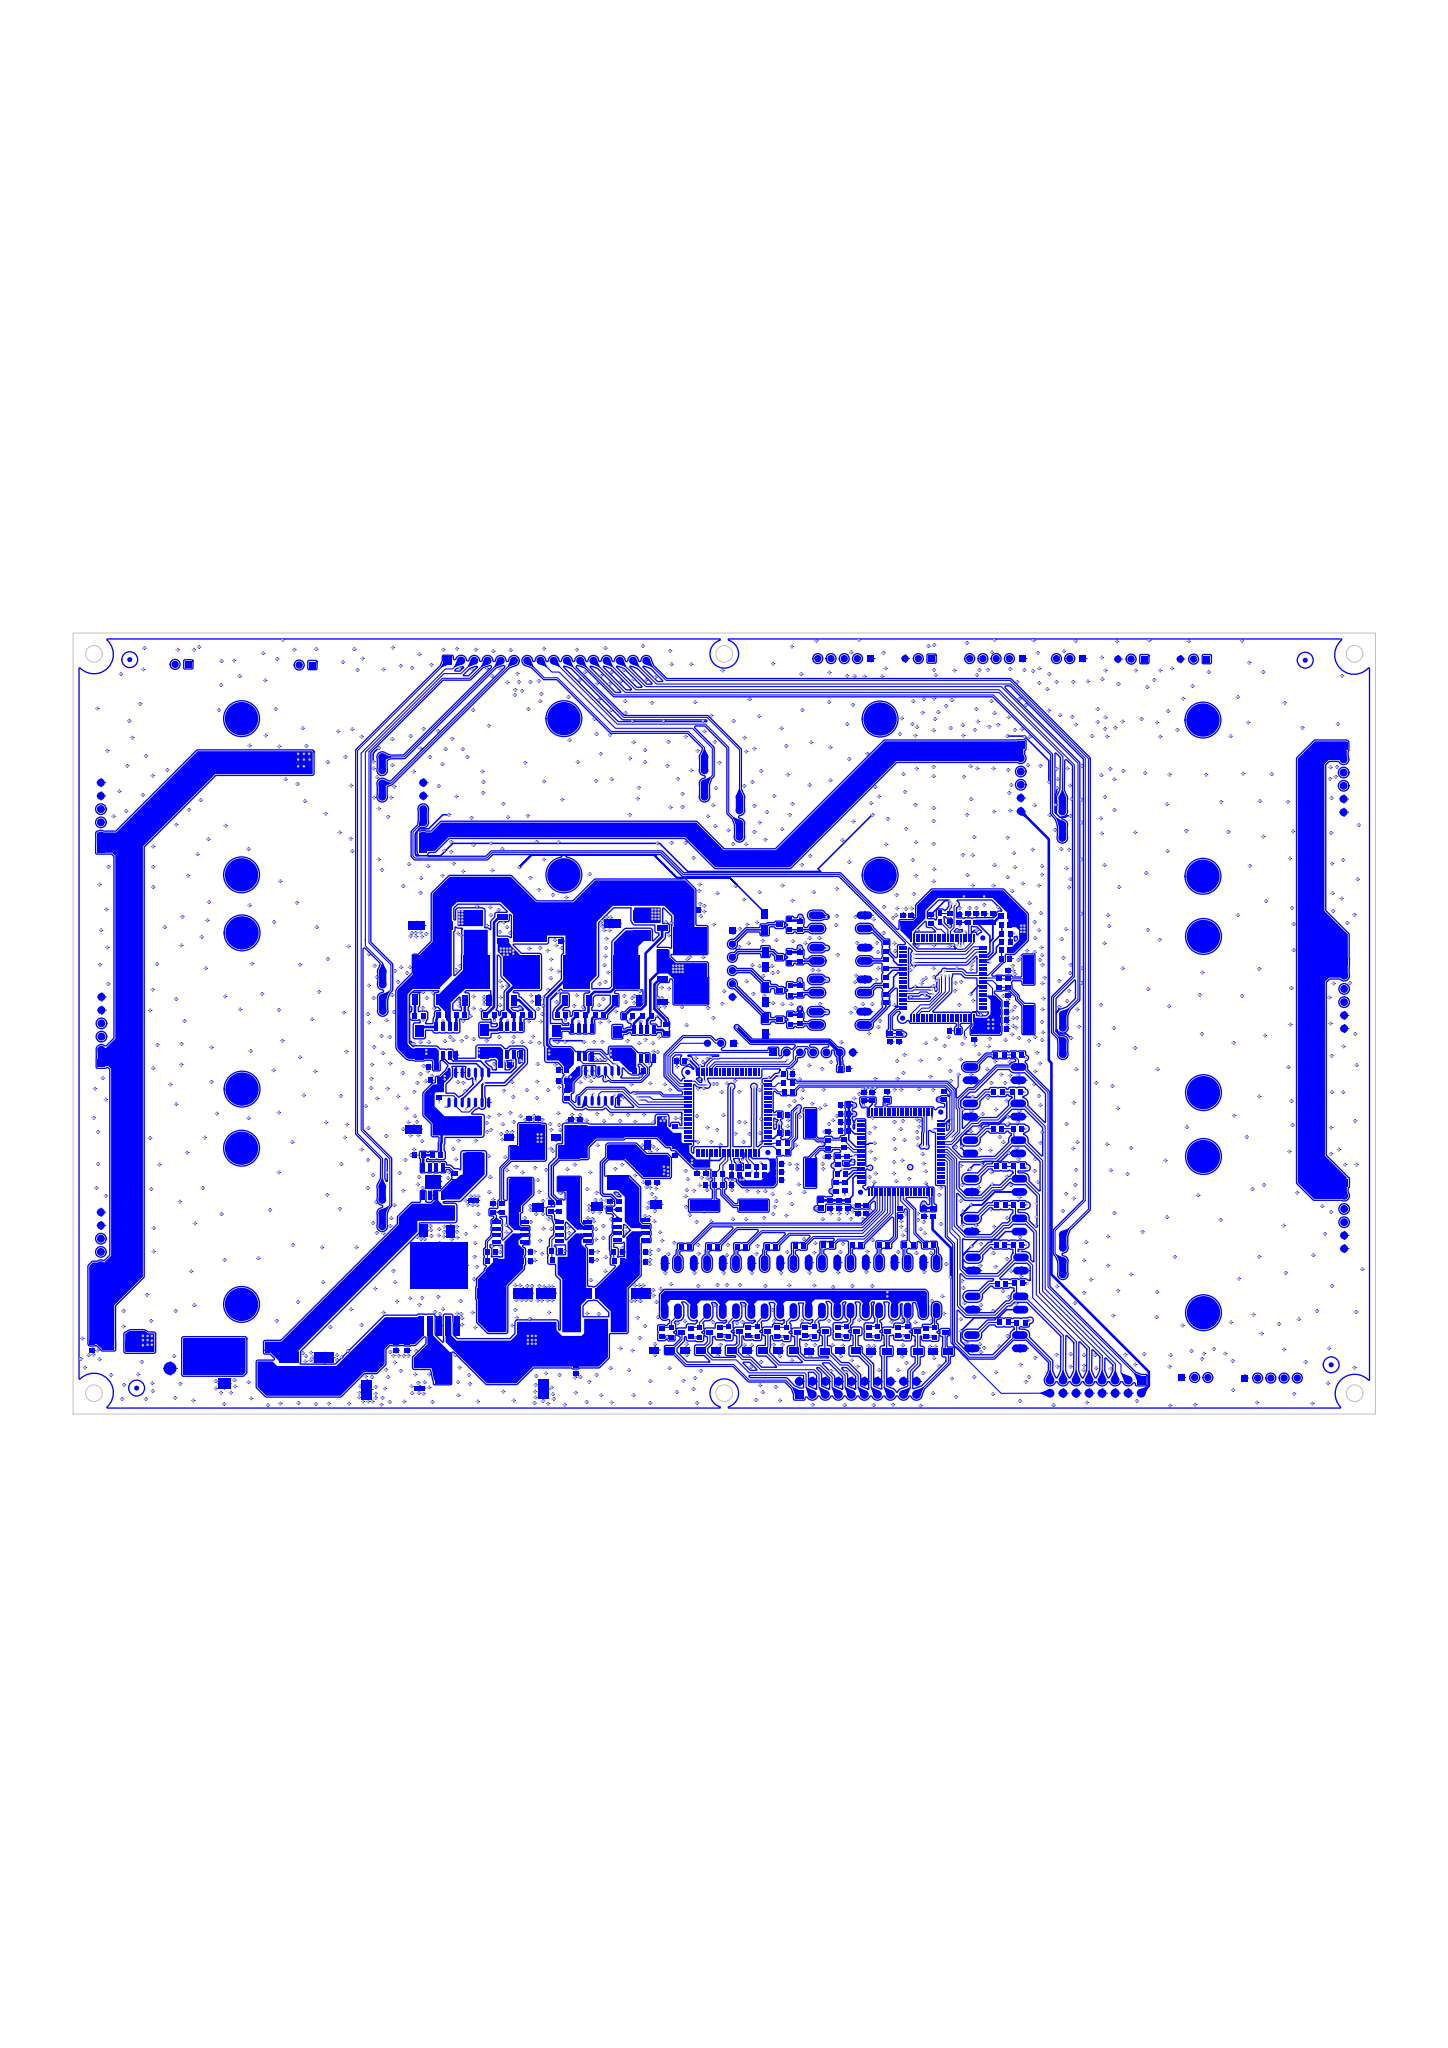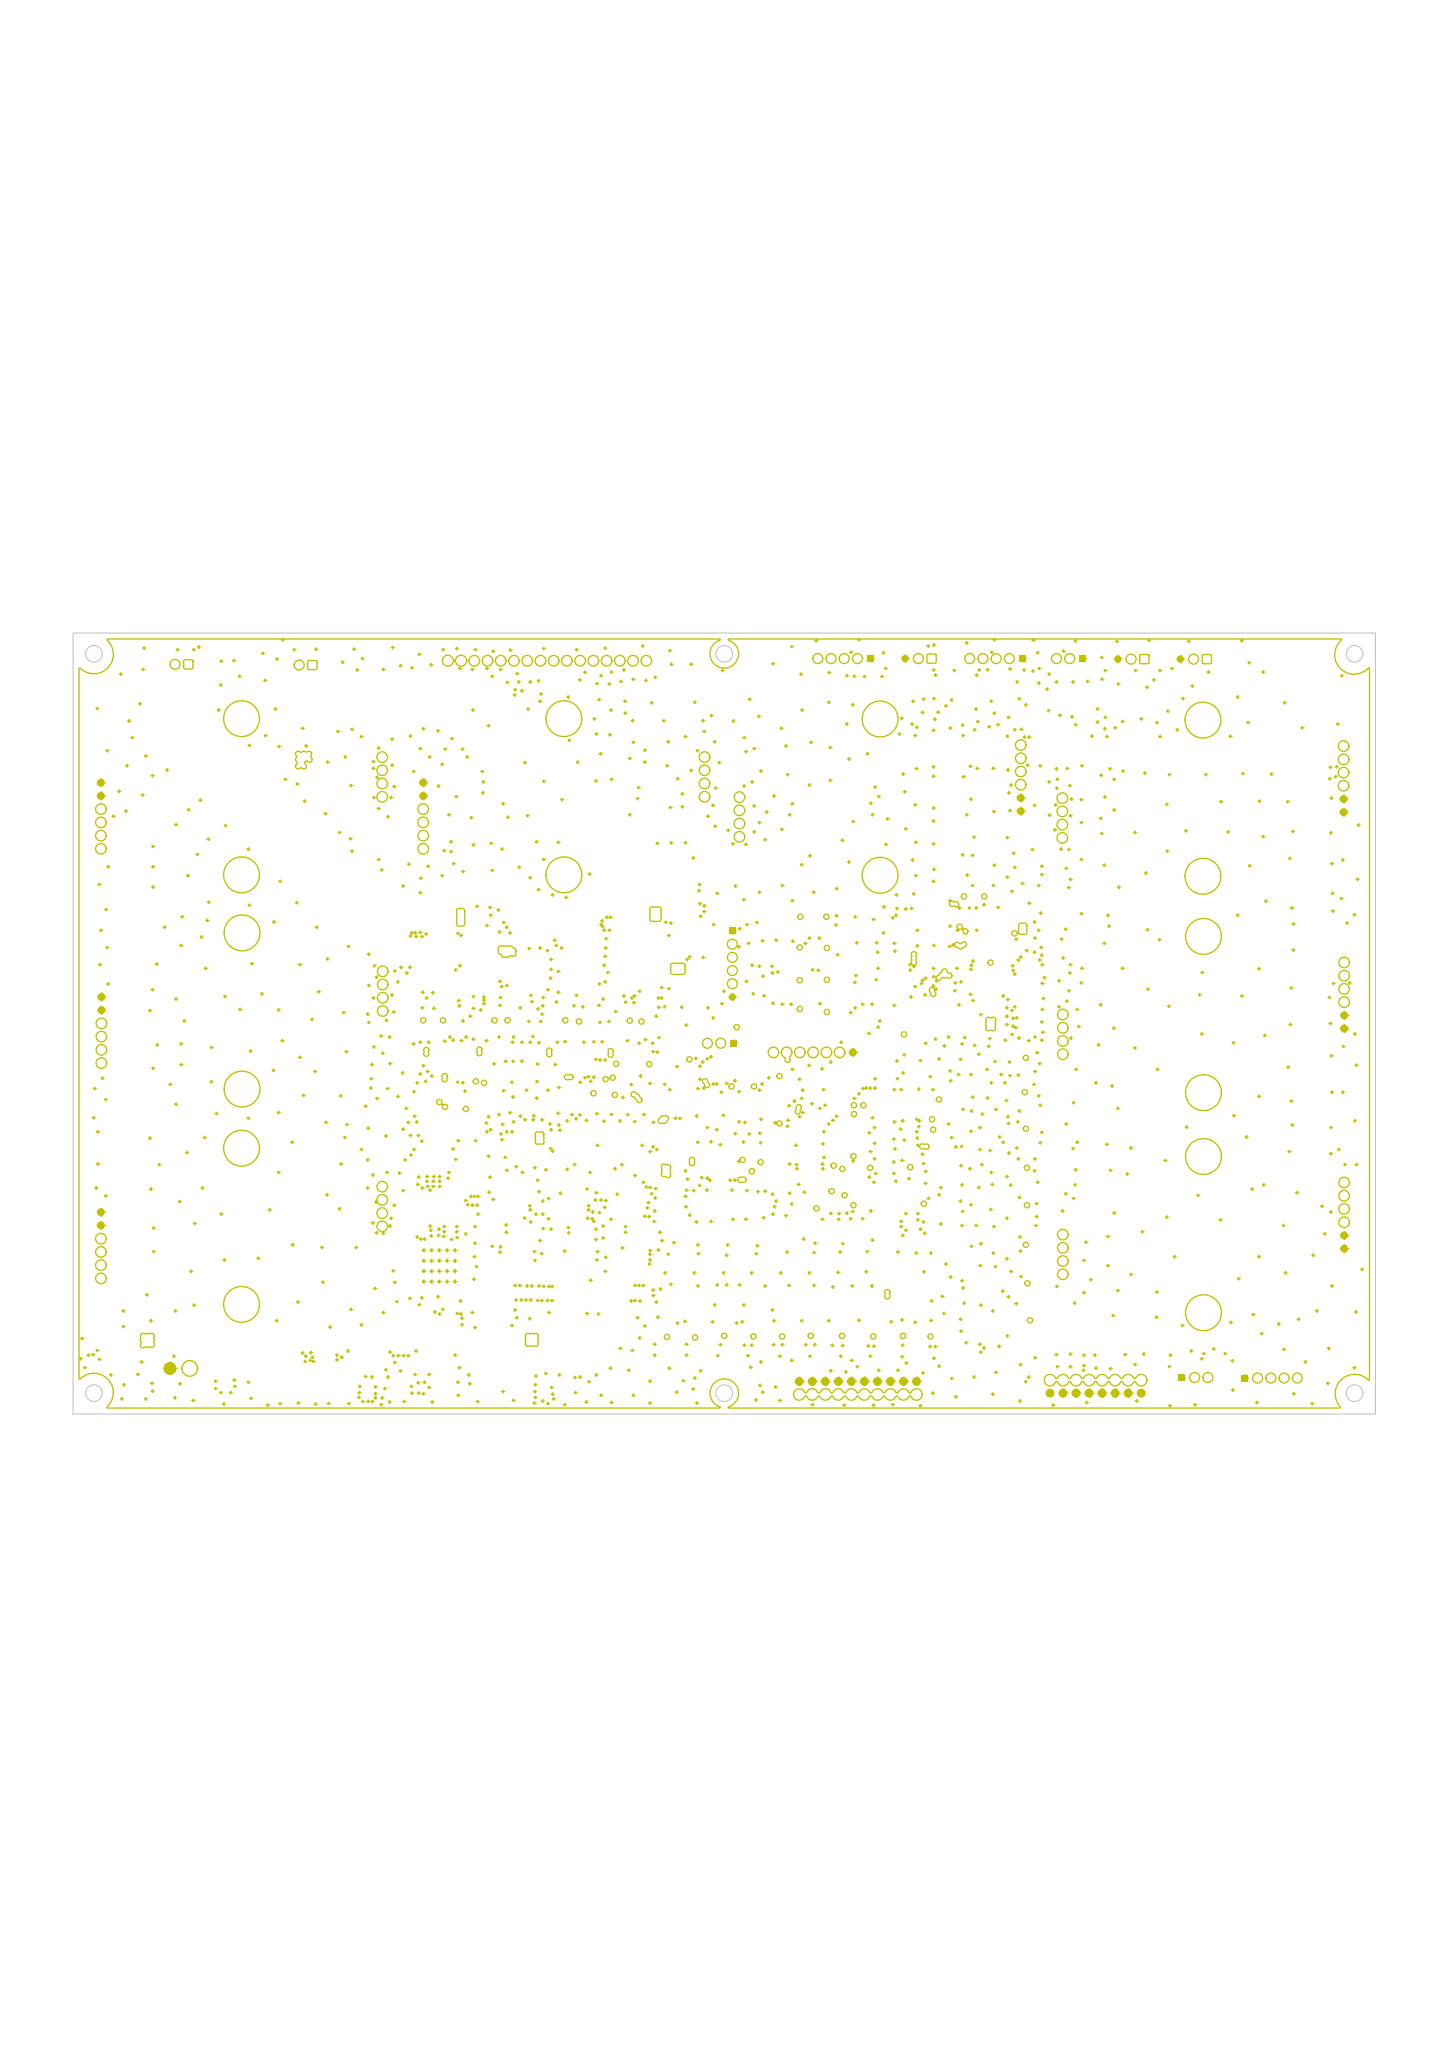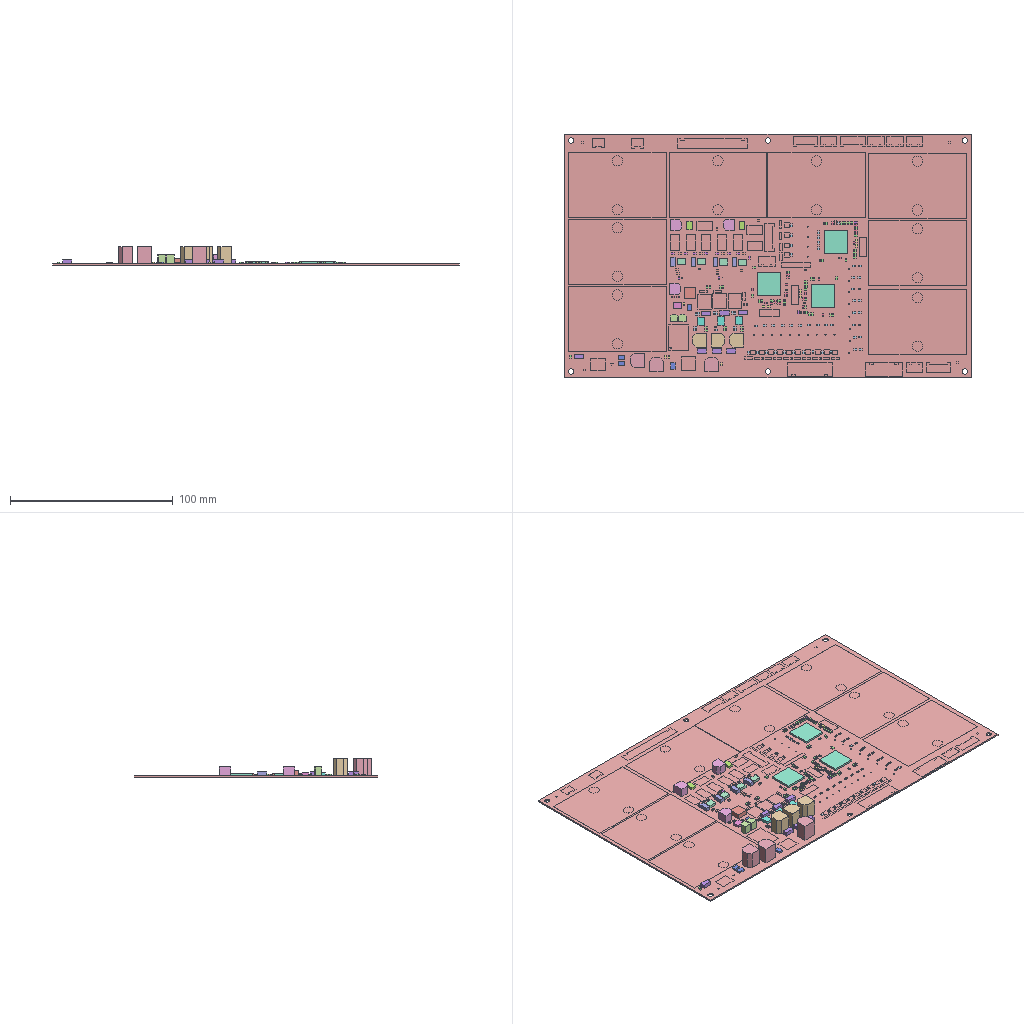Circuit board layout | Siemens PADS | box 250 x 150 x 11.4 mm
Layer stack:
layer,name,type,plane,layer_thickness_mm,copper_thickness_mm,dielectric_constant
0,,,,0,,3.3
1,Top,ROUTING,NONE,0.254,0.0343,4.3
2,Inner Layer 2,ROUTING,NONE,0.254,0.0343,4.3
3,Inner Layer 3,ROUTING,NONE,0.254,0.0343,4.3
4,Bottom,ROUTING,NONE,0,0.0343,3.3
Part placement:
Ref,PartType,Decal,X_mm,Y_mm,Rotation,Layer,Placed,Installed
C1,CAP_POL1,CAPAE830X1050N,56.395,8.15,270,Top,True,True
C2,CAP_POL1,CAPAE830X1050N,90.392,8.236,270,Top,True,True
C3,CAP_100NF_0805,C0603,110.293,45.172,90,Top,True,True
C4,CAP_100NF_0805,C0603,112.024,45.172,90,Top,True,True
C5,CAP3216,CAPAE830X1050N,82.871,23.207,0,Top,True,True
C6,CAP3216,3216,85.227,53.17,0,Top,True,True
C7,CAP_100NF_0805,C0603,89.203,55.978,270,Top,True,True
C8,CAP_100NF_0805,C0603,87.485,55.949,270,Top,True,True
C9,CAP_100NF_0805,C0603,86.921,31.17,180,Top,True,True
C10,CAP_100NF_0805,C0603,86.942,29.308,180,Top,True,True
C11,CAP3216,CAPAE830X1050N,94.232,23.207,180,Top,True,True
C12,CAP3216,3216,94.206,53.039,0,Top,True,True
C13,CAP_100NF_0805,C0603,97.278,55.851,270,Top,True,True
C14,CAP_100NF_0805,C0603,95.655,55.851,270,Top,True,True
C15,CAP_100NF_0805,C0603,98.736,31.121,180,Top,True,True
C16,CAP_100NF_0805,C0603,98.724,29.494,180,Top,True,True
C17,CAP_100NF_0805,C0603,131.981,47.469,0,Top,True,True
C18,CAP,C0603,61.963,13.017,90,Top,True,True
C19,CAP,C0603,64.165,12.988,90,Top,True,True
C20,CAP,C0603,96.464,8.581,90,Top,True,True
C21,CAP3216,CAPAE830X1050N,105.588,23.231,0,Top,True,True
C22,CAP_100NF_0805,C0603,109.049,29.24,180,Top,True,True
C23,CAP_100NF_0805,C0603,109.049,31.131,180,Top,True,True
C24,CAP3216,3216,110.244,50.174,270,Top,True,True
C25,CAP,C0603,73.389,45.447,90,Top,True,True
C26,CAP_POL1,CAPAE430X550N,72.408,36.917,270,Top,True,True
C27,CAP_POL1,CAPAE430X550N,67.231,36.99,270,Top,True,True
C28,CAP_POL1,CAPAE660X550N,68.037,54.705,180,Top,True,True
C29,CAP_100NF_0805,C0603,148.108,59.271,0,Top,True,True
C30,CAP_100NF_0805,C0603,151.754,60.975,270,Top,True,True
C31,CAP_100NF_0805,C0603,148.117,56.005,0,Top,True,True
C32,CAP_100NF_0805,C0603,164.982,38.757,90,Top,True,True
C33,CAP_100NF_0805,C0603,152.221,39.272,90,Top,True,True
C34,CAP_100NF_0805,C0603,178.382,78.817,180,Top,True,True
C35,CAP_100NF_0805,C0603,178.382,77.19,180,Top,True,True
C36,CAP_100NF_0805,C0603,170.139,95.232,270,Top,True,True
C37,CAP_100NF_0805,C0603,156.888,72.256,90,Top,True,True
C38,CAP_100NF_0805,C0603,160.932,95.012,270,Top,True,True
C39,CAP_100NF_0805,C0603,148.079,66.351,180,Top,True,True
C40,CAP_100NF_0805,C0603,115.49,50.503,90,Top,True,True
C41,CAP_100NF_0805,C0603,121.404,47.068,90,Top,True,True
C42,CAP_100NF_0805,C0603,119.71,47.068,270,Top,True,True
C43,CAP_POL1,CAPAE830X1050N,44.8,10.8,0,Top,True,True
C44,CAP_100NF_0805,C0603,3.695,12.993,90,Top,True,True
C45,CAP,C0603,122.275,43.938,180,Top,True,True
C46,CAP_POL1,CAPAE660X550N,68.679,93.81,180,Top,True,True
C47,CAPACITOR_ST,C0603,71.026,76.584,0,Top,True,True
C48,CAP,C0603,125.511,43.934,0,Top,True,True
C49,CAPACITOR_ST,C0603,83.688,76.637,180,Top,True,True
C50,CAPACITOR_ST,C0603,68.944,66.651,0,Top,True,True
C51,CAPACITOR_ST,C0603,82.895,66.941,180,Top,True,True
C52,CAP_100NF_0805,C0603,127.218,47.483,180,Top,True,True
C53,CAPACITOR_ST,C0603,93.7,91.6,270,Top,True,True
C54,CAP_100NF_0805,C0603,116.614,67.895,0,Top,True,True
C55,CAP_100NF_0805,C0603,135.183,48.075,180,Top,True,True
C56,CAP_100NF_0805,C0603,135.176,46.501,180,Top,True,True
C57,CAP_100NF_0805,C0603,135.166,44.932,180,Top,True,True
C58,CAP_100NF_0805,C0603,136.354,54.019,180,Top,True,True
C59,CAPACITOR_ST,C0603,69.486,64.112,180,Top,True,True
C60,CAP_POL1,CAPAE660X550N,100.794,94.206,0,Top,True,True
C61,CAPACITOR_ST,C0603,97.529,76.62,0,Top,True,True
C62,CAPACITOR_ST,C0603,110.153,76.424,180,Top,True,True
C63,CAPACITOR_ST,C0603,93.982,66.145,0,Top,True,True
C64,CAP_100NF_0805,C0603,137.211,65.229,180,Top,True,True
C65,CAPACITOR_ST,C0603,108.662,65.975,180,Top,True,True
C66,CAPACITOR_ST,C0603,119.2,96.8,0,Top,True,True
C67,CAPACITOR_ST,C0603,93.903,63.946,180,Top,True,True
C68,CAP3216,3216,132.76,94.515,270,Top,True,True
C69,CAP3216,3216,132.974,80.576,90,Top,True,True
C70,CAP3216,3216,132.908,87.304,90,Top,True,True
C71,CAP3216,3216,132.998,74.462,90,Top,True,True
C76,CAP_100NF_0805,C0603,179.075,92.266,0,Top,True,True
C77,CAP3216,3216,113.129,12.276,0,Top,True,True
C78,CAP3216,3216,119.03,12.253,0,Top,True,True
C79,CAP3216,3216,124.939,12.223,0,Top,True,True
C80,CAP3216,3216,130.94,12.148,0,Top,True,True
C81,CAP3216,3216,136.83,12.111,0,Top,True,True
C82,CAP3216,3216,142.784,12.101,0,Top,True,True
C83,CAP3216,3216,148.679,12.114,0,Top,True,True
C84,CAP3216,3216,154.643,12.074,0,Top,True,True
C85,CAP3216,3216,160.596,12.015,0,Top,True,True
C86,CAP3216,3216,166.499,11.967,0,Top,True,True
C87,CAP,C0603,144.967,50.237,270,Top,True,True
C88,CAP,C0603,145.003,53.417,90,Top,True,True
C89,CAP_100NF_0805,C0603,148.493,48.673,90,Top,True,True
C90,CAP_100NF_0805,C0603,148.103,54.423,180,Top,True,True
C91,CAP_100NF_0805,C0603,148.118,57.619,0,Top,True,True
C92,CAP_100NF_0805,C0603,150.615,39.26,90,Top,True,True
C93,CAP_100NF_0805,C0603,163.385,38.76,90,Top,True,True
C94,CAP_100NF_0805,C0603,153.395,60.953,270,Top,True,True
C95,CAP_100NF_0805,C0603,167.261,61.215,270,Top,True,True
C96,CAP_100NF_0805,C0603,148.107,43.672,270,Top,True,True
C97,CAP_100NF_0805,C0603,145.385,40.226,90,Top,True,True
C98,CAP_100NF_0805,C0603,147.018,40.226,90,Top,True,True
C99,CAP_100NF_0805,C0603,148.703,40.226,90,Top,True,True
C107,CAP_100NF_0805,C0603,172.965,72.653,90,Top,True,True
C108,CAP_100NF_0805,C0603,178.373,75.595,180,Top,True,True
C109,CAP_100NF_0805,C0603,178.382,74.015,0,Top,True,True
C110,CAP,C0603,179.486,81.197,270,Top,True,True
C111,CAP,C0603,179.47,84.37,90,Top,True,True
C115,CAP_100NF_0805,C0603,179.039,87.464,180,Top,True,True
C116,CAP_100NF_0805,C0603,158.525,72.256,90,Top,True,True
C119,CAP_100NF_0805,C0603,173.356,95.246,270,Top,True,True
C120,CAP_100NF_0805,C0603,174.946,95.246,270,Top,True,True
C121,CAP_100NF_0805,C0603,176.536,95.256,270,Top,True,True
C124,CAP_100NF_0805,C0603,171.756,95.245,270,Top,True,True
C125,CAP_100NF_0805,C0603,159.307,95.02,270,Top,True,True
CN12,DEF_S_6,XH2.54-6PM,126.551,92.786,270,Top,True,True
D1,DIODE_18TQ045,SOD4725X110N,34.921,8.931,180,Top,True,True
D2,SMBJ50CA,DO-214AA,28.977,5.813,180,Top,True,True
D3,DIODE,SMA_1,84.24,16.651,0,Top,True,True
D4,DIODE_18TQ045,SOD4725X110N,76.884,43.351,270,Top,True,True
D5,DIODE,SMA_1,87.097,39.688,0,Top,True,True
D6,DIODE,SMA_1,93.399,16.656,180,Top,True,True
D7,DIODE,SMA_1,98.286,39.906,0,Top,True,True
D8,DIODE_18TQ045,SOD4725X110N,34.931,12.761,180,Top,True,True
D9,DIODE,SMA_1,8.98,13.153,0,Top,True,True
D10,DIODE02,SMA,66.464,71.391,270,Top,True,True
D11,DIODE02,SMA,79.061,71.539,270,Top,True,True
D12,DIODE02,SMA,92.746,71.278,270,Top,True,True
D13,DIODE02,SMA,104.475,71.216,270,Top,True,True
D14,DIODE,SMA_1,102.359,16.575,180,Top,True,True
D16,DIODE,SMA_1,109.663,40.216,0,Top,True,True
D21,DIODE_18TQ045,SOD4725X110N,66.517,7.314,270,Top,True,True
F1,FUSE,5032X150N,76.71,93.864,90,Top,True,True
F2,FUSE,5032X150N,109.133,93.856,90,Top,True,True
J1,MHDR1X2,DEF_KF2EDG_381_180D,20.498,11.755,180,Top,True,True
J2,DEF_S_16,XH2.54-16P,71.933,144.678,0,Top,True,True
J3,CON3_2,XH2.54-3PM,205.638,144.983,180,Top,True,True
J4,CON7,SIP-7P,134.44,69.45,0,Top,True,True
J5,HEADER_5,XH2.54-5PM,153.111,145.085,180,Top,True,True
J6,CON3_2,XH2.54-3PM,217.627,144.983,180,Top,True,True
J7,DEF_D_16,XHD_2.5_16P,205.029,6.502,180,Top,True,True
J8,CON3,XH2.54-3PM,126.852,71.206,180,Top,True,True
J9,MHDR1X2,XH2.54-2PM,22.122,143.98,180,Top,True,True
J10,MHDR1X2,XH2.54-2PM,45.94,143.846,180,Top,True,True
J11,CON3_2,XH2.54-3PM,164.795,145.085,180,Top,True,True
J14,CON3,XH2.54-3PM,193.853,145.085,180,Top,True,True
J20,HEADER_5,XH2.54-5PM,224.841,6.909,0,Top,True,True
J21,CON3,XH2.54-3PM,212.75,7.01,0,Top,True,True
JP1,HEADER_5,XH2.54-5PM,182.27,145.085,180,Top,True,True
JT5,DEF_D_20,XHD_2.5_20P,139.395,3.759,0,Top,True,True
L1,IND-MOLDED,L7.5_7.5,104.656,47.297,270,Top,True,True
L2,INDUCTOR,L7X7,77.052,52.43,90,Top,True,True
L4,IND-MOLDED,L7.5_7.5,86.05,46.968,270,Top,True,True
L5,INDUCTOR,L12_12,76.115,8.837,180,Top,True,True
L6,IND-MOLDED,L7.5_7.5,95.271,47.187,270,Top,True,True
L11,INDUCTOR,L0603,178.987,95.677,180,Top,True,True
L12,INDUCTOR,L0603,143.648,40.278,90,Top,True,True
R1,RES1,R0603,69.794,49.718,180,Top,True,True
R2,RES1,R0603,66.413,49.718,180,Top,True,True
R3,RESISTOR_ST,R0603,66.426,76.496,180,Top,True,True
R4,RESISTOR_ST,R0603,74.379,76.67,0,Top,True,True
R5,RESISTOR_ST,R0603,80.058,76.609,0,Top,True,True
R6,RES1,R0603,123.944,46.049,180,Top,True,True
R7,RES1,R0603,136.37,57.437,0,Top,True,True
R8,RESISTOR_ST,R0603,87.096,76.692,180,Top,True,True
R9,RESISTOR_ST,R0603,70.303,61.569,270,Top,True,True
R10,RES1,R0603,127.183,45.904,0,Top,True,True
R11,RES1,R0603,115.581,54.377,90,Top,True,True
R12,RES1,R0603,129.574,46.722,90,Top,True,True
R13,RES0603,R0603,104.697,40.07,90,Top,True,True
R14,RES0603,R0603,103.087,40.007,90,Top,True,True
R15,RES0603,R0603,92.758,29.631,180,Top,True,True
R16,RES0603,R0603,92.709,31.324,0,Top,True,True
R17,RES0603,R0603,93.299,39.754,90,Top,True,True
R18,RES0603,R0603,91.723,39.737,90,Top,True,True
R19,RES1,R0603,136.25,52.028,180,Top,True,True
R20,RES1,R0603,136.264,50.315,180,Top,True,True
R21,RES1,R0603,137.26,63.543,180,Top,True,True
R22,RES1,R0603,137.309,61.877,180,Top,True,True
R23,RESISTOR_ST,R0603,93.74,76.62,180,Top,True,True
R24,RESISTOR_ST,R0603,101.1,76.62,0,Top,True,True
R25,RESISTOR_ST,R0603,106.671,76.477,0,Top,True,True
R26,RESISTOR_ST,R0603,113.763,73.915,270,Top,True,True
R27,RESISTOR_ST,R0603,94.881,61.42,270,Top,True,True
R28,RES0603,R0603,156.026,89.702,270,Top,True,True
R29,RES0603,R0603,139.564,93.827,90,Top,True,True
R30,RES0603,R0603,155.971,83.109,90,Top,True,True
R31,RES0603,R0603,139.549,81.427,90,Top,True,True
R32,RES0603,R0603,104.633,29.358,180,Top,True,True
R33,RES0603,R0603,104.587,31.12,0,Top,True,True
R34,RES1,R0603,179.017,93.903,0,Top,True,True
R35,RES1,R0603,169.122,73.638,0,Top,True,True
R36,RES1,R0603,164.634,95.082,270,Top,True,True
R37,RES0603,R0603,177.529,61.839,0,Top,True,True
R38,RES0603,R0603,181.254,54.807,0,Top,True,True
R39,RES0603,R0603,178.086,47.55,0,Top,True,True
R40,RES0603,R0603,181.393,47.55,0,Top,True,True
R41,RES0603,R0603,178.112,40.096,0,Top,True,True
R42,RES0603,R0603,181.376,40.118,0,Top,True,True
R43,RES0603,R0603,177.997,32.538,0,Top,True,True
R44,RES0603,R0603,181.273,32.523,0,Top,True,True
R45,RES1,R0603,146.427,43.629,270,Top,True,True
R46,RES1,R0603,156.292,61.057,270,Top,True,True
R47,RES1,R0603,148.001,51.965,90,Top,True,True
R48,RES1,R0603,146.83,48.637,270,Top,True,True
R49,RES1,R0603,158.785,38.665,90,Top,True,True
R50,RES1,R0603,147.468,46.049,0,Top,True,True
R51,RES0603,R0603,117.518,32.084,0,Top,True,True
R52,RES0603,R0603,112.962,15.605,270,Top,True,True
R53,RES0603,R0603,122.942,32.127,0,Top,True,True
R54,RES0603,R0603,118.583,15.662,270,Top,True,True
R55,RES0603,R0603,128.325,32.168,0,Top,True,True
R56,RES0603,R0603,124.129,15.877,270,Top,True,True
R57,RES0603,R0603,134.108,32.156,0,Top,True,True
R58,RES0603,R0603,129.608,15.84,270,Top,True,True
R59,RES0603,R0603,139.398,32.208,0,Top,True,True
R60,RES0603,R0603,135.162,15.728,270,Top,True,True
R61,RES0603,R0603,144.863,32.404,0,Top,True,True
R62,RES0603,R0603,140.567,15.825,270,Top,True,True
R63,RES0603,R0603,150.37,32.507,0,Top,True,True
R64,RES0603,R0603,146.76,15.891,270,Top,True,True
R65,RES0603,R0603,155.623,32.515,0,Top,True,True
R66,RES0603,R0603,152.714,15.845,270,Top,True,True
R67,RES0603,R0603,160.477,32.477,0,Top,True,True
R68,RES0603,R0603,158.404,15.814,270,Top,True,True
R69,RES0603,R0603,164.368,32.438,180,Top,True,True
R70,RES0603,R0603,163.759,15.709,270,Top,True,True
R71,RES0603,R0603,177.947,68.974,0,Top,True,True
R72,RES0603,R0603,181.332,68.974,0,Top,True,True
R73,RES1,R0603,177.81,82.755,270,Top,True,True
R74,RES0603,R0603,181.159,61.892,0,Top,True,True
R75,RES0603,R0603,177.422,54.815,0,Top,True,True
R76,RES1,R0603,179.018,89.062,0,Top,True,True
R77,RES1,R0603,131.961,45.844,0,Top,True,True
R78,RES1,R0603,179.055,90.694,180,Top,True,True
R79,RES0603,R0603,80.329,29.356,180,Top,True,True
R80,RES0603,R0603,80.329,31.094,0,Top,True,True
R81,RES0603,R0603,82.278,39.557,90,Top,True,True
R82,RES0603,R0603,80.585,39.577,90,Top,True,True
R83,RES0603,R0603,178.225,25.034,0,Top,True,True
R84,RES0603,R0603,181.533,25.104,0,Top,True,True
R85,RES0603,R0603,178.664,17.584,0,Top,True,True
R86,RES0603,R0603,181.935,17.566,0,Top,True,True
R87,RES0603,R0603,156.024,86.449,270,Top,True,True
R88,RES0603,R0603,139.555,87.79,90,Top,True,True
R89,RES0603,R0603,156.036,79.756,90,Top,True,True
R90,RES0603,R0603,139.547,75.749,90,Top,True,True
R91,RES0603,R0603,168.271,95.3,90,Top,True,True
R92,RES0603,0603,166.462,95.343,270,Top,True,True
U1,LM2596,LM2596,70.279,16.963,0,Top,True,True
U2,DEF_TD1410,SOIC127P600X175-8N,107.212,35.378,180,Top,True,True
U3,DEF_TD1410,SOIC127P600X175-8N,96.081,35.043,180,Top,True,True
U4,DEF_HART_MD,DEF_HART_MD,2.337,16.053,0,Top,True,True
U5,TPS5430,SOIC127P600X175-9N,69.104,44.638,270,Top,True,True
U6,DEF_HART_MD,DEF_HART_MD,2.438,57.404,0,Top,True,True
U7,DEF_HART_MD,DEF_HART_MD,2.337,98.552,0,Top,True,True
U8,DEF_HART_MD,DEF_HART_MD,64.211,98.552,0,Top,True,True
U9,DEF_HART_MD,DEF_HART_MD,184.912,138.481,180,Top,True,True
U10,STM32F103VCT6,QFP50P1600X1600X120-100N,125.683,57.923,90,Top,True,True
U11,PC817,SO4M1,164.473,24.478,180,Top,True,True
U12,AO3415-2,SOT23,115.83,15.691,270,Top,True,True
U13,PC817,SO4M1,114.834,24.323,180,Top,True,True
U14,AO3415-2,SOT23,121.209,15.687,270,Top,True,True
U15,PC817,SO4M1,120.428,24.363,180,Top,True,True
U16,AO3415-2,SOT23,126.85,15.84,270,Top,True,True
U17,PC817,SO4M1,125.979,24.356,180,Top,True,True
U18,AO3415-2,SOT23,132.329,15.877,270,Top,True,True
U19,PC817,SO4M1,131.472,24.356,180,Top,True,True
U20,AO3415-2,SOT23,137.958,15.691,270,Top,True,True
U21,PC817,SO4M1,137.007,24.396,180,Top,True,True
U22,AO3415-2,SOT23,143.397,15.848,270,Top,True,True
U23,PC817,SO4M1,142.476,24.468,180,Top,True,True
U24,AO3415-2,SOT23,149.386,15.885,270,Top,True,True
U25,PC817,SO4M1,147.961,24.468,180,Top,True,True
U26,AO3415-2,SOT23,155.367,15.875,270,Top,True,True
U27,PC817,SO4M1,153.443,24.504,180,Top,True,True
U28,AO3415-2,SOT23,161.084,15.824,270,Top,True,True
U29,PC817,SO4M1,158.94,24.504,180,Top,True,True
U30,AO3415-2,SOT23,166.363,15.725,270,Top,True,True
U31,STM32F103VCT6,QFP50P1600X1600X120-100N,166.931,83.734,180,Top,True,True
U32,PC817,SO4M1,176.888,65.382,270,Top,True,True
U33,PC817,SO4M1,176.826,58.381,270,Top,True,True
U34,DEF_TD1410,SOIC127P600X175-8N,83.952,34.975,180,Top,True,True
U35,PC817,SO4M1,176.862,51.318,270,Top,True,True
U36,PC817,SO4M1,177.05,43.918,270,Top,True,True
U37,PC817,SO4M1,177.069,36.306,270,Top,True,True
U38,PC817,SO4M1,177.356,28.806,270,Top,True,True
U39,PC817,SO4M1,177.286,21.311,270,Top,True,True
U40,PC817,SO4M1,177.138,13.895,270,Top,True,True
U41,STM32F103VCT6,QFP50P1600X1600X120-100N,158.853,50.289,0,Top,True,True
U42,DEF_HART_MD,DEF_HART_MD,246.888,138.278,180,Top,True,True
U43,DEF_HART_MD,DEF_HART_MD,246.99,96.723,180,Top,True,True
U44,DEF_HART_MD,DEF_HART_MD,246.99,54.458,180,Top,True,True
U45,DEF_IR2104S,SOIC127P600X175-8N,71.653,71.632,90,Top,True,True
U46,DEF_IR2104S,SOIC127P600X175-8N,84.004,71.718,90,Top,True,True
U47,MC74HC00A,SO14NB,75.971,62.701,0,Top,True,True
U48,DEF_IR2104S,SOIC127P600X175-8N,97.715,71.309,90,Top,True,True
U49,DEF_IR2104S,SOIC127P600X175-8N,109.558,71.059,90,Top,True,True
U50,MC74HC00A,SO14NB,100.908,63.025,0,Top,True,True
U51,AO3415-2,SOT23,136.617,93.951,90,Top,True,True
U52,PC817,SO4M1,147.316,94.513,90,Top,True,True
U53,AO3415-2,SOT23,136.629,81.389,90,Top,True,True
U54,PC817,SO4M1,147.316,82.205,90,Top,True,True
U55,AO3415-2,SOT23,136.611,87.736,90,Top,True,True
U56,PC817,SO4M1,147.386,88.289,90,Top,True,True
U57,AO3415-2,SOT23,136.702,75.731,90,Top,True,True
U58,PC817,SO4M1,147.261,75.997,90,Top,True,True
U59,MARK,MARK,241.503,9.449,0,Top,True,True
U60,MARK,MARK,236.525,144.78,0,Top,True,True
U61,MARK,MARK,10.871,144.882,0,Top,True,True
U62,MARK,MARK,12.192,4.978,0,Top,True,True
VT1,DEF_IRF540NS,DPAK4-4,67.912,81.069,0,Top,True,True
VT2,DEF_IRF540NS,DPAK4-4,77.473,81.056,0,Top,True,True
VT3,DEF_IRF540NS,DPAK4-4,83.895,93.176,270,Top,True,True
VT4,DEF_IRF540NS,DPAK4-4,87.006,81.064,0,Top,True,True
VT5,DEF_IRF540NS,DPAK4-4,96.655,81.013,0,Top,True,True
VT6,DEF_IRF540NS,DPAK4-4,106.311,81.018,0,Top,True,True
VT7,DEF_IRF540NS,DPAK4-4,114.626,91.023,270,Top,True,True
VT8,DEF_IRF540NS,DPAK4-4,114.775,81.349,270,Top,True,True
X1,XTAL,DEF_49S_MD,125.878,42.32,180,Top,True,True
X2,XTAL,DEF_49S_MD,181.087,80.615,270,Top,True,True
X3,XTAL,DEF_49S_MD,143.775,51.088,90,Top,True,True
Pad and via stacks:
via_name,drill_mm,start_layer,end_layer,type,pad_size_top,pad_size_inner,pad_size_bottom
JMPVIA_AAAAA,0.9398,1,4,through,1.397,1.778,1.397
1-4,0.2499,1,4,through,0.5001,0.5001,0.5001
Design rules, without the lines most boards share, first 368 of 3527 lines:
# PADS Layout design rules of , as PADS writes them (units: mils, PADS database units)
THERLINEWID 15
THERSMDWID 10
THERFLAGS 1044735
HATCHGRID 4
MINHATAREA 0
HATCHMODE 0
DRILLHOLE 6
DRLOVERSIZE 3
VIAMODE A
LAYERPAIR 1      2
TEARDROP 7563354
RULES_SECTION MILS
{
NET_CLASS DATA
GROUP DATA
ASSOCIATED_NET DATA
DESIGN RULES
{
RULE_SET (1)
{
FOR :
{
DEFAULT :
}
AGAINST :
{
DEFAULT :
}
LAYER 0
CLEARANCE_RULE :
{
TRACK_TO_TRACK 8
VIA_TO_TRACK 8
VIA_TO_VIA 8
PAD_TO_TRACK 8
PAD_TO_VIA 10
PAD_TO_PAD 6
SMD_TO_TRACK 8
SMD_TO_VIA 8
SMD_TO_PAD 6
SMD_TO_SMD 6
COPPER_TO_TRACK 10
COPPER_TO_VIA 10
COPPER_TO_PAD 10
COPPER_TO_SMD 10
COPPER_TO_COPPER 8
TEXT_TO_TRACK 8
TEXT_TO_VIA 8
TEXT_TO_PAD 6
TEXT_TO_SMD 6
OUTLINE_TO_TRACK 40
OUTLINE_TO_VIA 40
OUTLINE_TO_PAD 10
OUTLINE_TO_SMD 10
OUTLINE_TO_COPPER 40
DRILL_TO_TRACK 8
DRILL_TO_VIA 8
DRILL_TO_PAD 8
DRILL_TO_SMD 8
DRILL_TO_COPPER 8
SAME_NET_SMD_TO_VIA 0
SAME_NET_SMD_TO_CRN 0
SAME_NET_VIA_TO_VIA 0
SAME_NET_PAD_TO_CRN 0
MIN_TRACK_WIDTH 8
REC_TRACK_WIDTH 8
MAX_TRACK_WIDTH 196.85
DRILL_TO_DRILL 6
BODY_TO_BODY 6
SAME_NET_TRACK_TO_CRN 0
}
}
RULE_SET (2)
{
FOR :
{
NET VCC_3V3_A
}
AGAINST :
{
DEFAULT :
}
LAYER 0
CLEARANCE_RULE :
{
TRACK_TO_TRACK 5.91
VIA_TO_TRACK 5.91
VIA_TO_VIA 5.91
PAD_TO_TRACK 5.91
PAD_TO_VIA 5.91
PAD_TO_PAD 5.91
SMD_TO_TRACK 5.91
SMD_TO_VIA 5.91
SMD_TO_PAD 5.91
SMD_TO_SMD 5.91
COPPER_TO_TRACK 5.91
COPPER_TO_VIA 5.91
COPPER_TO_PAD 5.91
COPPER_TO_SMD 5.91
COPPER_TO_COPPER 5.91
TEXT_TO_TRACK 5.91
TEXT_TO_VIA 5.91
TEXT_TO_PAD 5.91
TEXT_TO_SMD 5.91
OUTLINE_TO_TRACK 5.91
OUTLINE_TO_VIA 5.91
OUTLINE_TO_PAD 5.91
OUTLINE_TO_SMD 5.91
OUTLINE_TO_COPPER 5.91
DRILL_TO_TRACK 5.91
DRILL_TO_VIA 5.91
DRILL_TO_PAD 5.91
DRILL_TO_SMD 5.91
DRILL_TO_COPPER 5.91
SAME_NET_SMD_TO_VIA 0
SAME_NET_SMD_TO_CRN 0
SAME_NET_VIA_TO_VIA 0
SAME_NET_PAD_TO_CRN 0
MIN_TRACK_WIDTH 5.91
REC_TRACK_WIDTH 11.81
MAX_TRACK_WIDTH 196.85
DRILL_TO_DRILL 5.91
BODY_TO_BODY 5.91
SAME_NET_TRACK_TO_CRN 0
}
}
RULE_SET (3)
{
FOR :
{
NET V-A2
}
AGAINST :
{
DEFAULT :
}
LAYER 0
CLEARANCE_RULE :
{
TRACK_TO_TRACK 5.91
VIA_TO_TRACK 5.91
VIA_TO_VIA 5.91
PAD_TO_TRACK 5.91
PAD_TO_VIA 5.91
PAD_TO_PAD 5.91
SMD_TO_TRACK 5.91
SMD_TO_VIA 5.91
SMD_TO_PAD 5.91
SMD_TO_SMD 5.91
COPPER_TO_TRACK 5.91
COPPER_TO_VIA 5.91
COPPER_TO_PAD 5.91
COPPER_TO_SMD 5.91
COPPER_TO_COPPER 5.91
TEXT_TO_TRACK 5.91
TEXT_TO_VIA 5.91
TEXT_TO_PAD 5.91
TEXT_TO_SMD 5.91
OUTLINE_TO_TRACK 5.91
OUTLINE_TO_VIA 5.91
OUTLINE_TO_PAD 5.91
OUTLINE_TO_SMD 5.91
OUTLINE_TO_COPPER 5.91
DRILL_TO_TRACK 5.91
DRILL_TO_VIA 5.91
DRILL_TO_PAD 5.91
DRILL_TO_SMD 5.91
DRILL_TO_COPPER 5.91
SAME_NET_SMD_TO_VIA 0
SAME_NET_SMD_TO_CRN 0
SAME_NET_VIA_TO_VIA 0
SAME_NET_PAD_TO_CRN 0
MIN_TRACK_WIDTH 5.91
REC_TRACK_WIDTH 19.69
MAX_TRACK_WIDTH 196.85
DRILL_TO_DRILL 5.91
BODY_TO_BODY 5.91
SAME_NET_TRACK_TO_CRN 0
}
}
RULE_SET (4)
{
FOR :
{
NET $$$715
}
AGAINST :
{
DEFAULT :
}
LAYER 0
CLEARANCE_RULE :
{
TRACK_TO_TRACK 5.91
VIA_TO_TRACK 5.91
VIA_TO_VIA 5.91
PAD_TO_TRACK 5.91
PAD_TO_VIA 5.91
PAD_TO_PAD 5.91
SMD_TO_TRACK 5.91
SMD_TO_VIA 5.91
SMD_TO_PAD 5.91
SMD_TO_SMD 5.91
COPPER_TO_TRACK 5.91
COPPER_TO_VIA 5.91
COPPER_TO_PAD 5.91
COPPER_TO_SMD 5.91
COPPER_TO_COPPER 5.91
TEXT_TO_TRACK 5.91
TEXT_TO_VIA 5.91
TEXT_TO_PAD 5.91
TEXT_TO_SMD 5.91
OUTLINE_TO_TRACK 5.91
OUTLINE_TO_VIA 5.91
OUTLINE_TO_PAD 5.91
OUTLINE_TO_SMD 5.91
OUTLINE_TO_COPPER 5.91
DRILL_TO_TRACK 5.91
DRILL_TO_VIA 5.91
DRILL_TO_PAD 5.91
DRILL_TO_SMD 5.91
DRILL_TO_COPPER 5.91
SAME_NET_SMD_TO_VIA 0
SAME_NET_SMD_TO_CRN 0
SAME_NET_VIA_TO_VIA 0
SAME_NET_PAD_TO_CRN 0
MIN_TRACK_WIDTH 5.91
REC_TRACK_WIDTH 11.81
MAX_TRACK_WIDTH 196.85
DRILL_TO_DRILL 5.91
BODY_TO_BODY 5.91
SAME_NET_TRACK_TO_CRN 0
}
}
RULE_SET (5)
{
FOR :
{
NET $$$719
}
AGAINST :
{
DEFAULT :
}
LAYER 0
CLEARANCE_RULE :
{
TRACK_TO_TRACK 5.91
VIA_TO_TRACK 5.91
VIA_TO_VIA 5.91
PAD_TO_TRACK 5.91
PAD_TO_VIA 5.91
PAD_TO_PAD 5.91
SMD_TO_TRACK 5.91
SMD_TO_VIA 5.91
SMD_TO_PAD 5.91
SMD_TO_SMD 5.91
COPPER_TO_TRACK 5.91
COPPER_TO_VIA 5.91
COPPER_TO_PAD 5.91
COPPER_TO_SMD 5.91
COPPER_TO_COPPER 5.91
TEXT_TO_TRACK 5.91
TEXT_TO_VIA 5.91
TEXT_TO_PAD 5.91
TEXT_TO_SMD 5.91
OUTLINE_TO_TRACK 5.91
OUTLINE_TO_VIA 5.91
OUTLINE_TO_PAD 5.91
OUTLINE_TO_SMD 5.91
OUTLINE_TO_COPPER 5.91
DRILL_TO_TRACK 5.91
DRILL_TO_VIA 5.91
DRILL_TO_PAD 5.91
DRILL_TO_SMD 5.91
DRILL_TO_COPPER 5.91
SAME_NET_SMD_TO_VIA 0
SAME_NET_SMD_TO_CRN 0
SAME_NET_VIA_TO_VIA 0
SAME_NET_PAD_TO_CRN 0
MIN_TRACK_WIDTH 5.91
REC_TRACK_WIDTH 11.81
MAX_TRACK_WIDTH 196.85
DRILL_TO_DRILL 5.91
BODY_TO_BODY 5.91
SAME_NET_TRACK_TO_CRN 0
}
}
RULE_SET (6)
{
FOR :
{
NET M2-
}
AGAINST :
{
DEFAULT :
}
LAYER 0
CLEARANCE_RULE :
{
TRACK_TO_TRACK 5.91
VIA_TO_TRACK 5.91
VIA_TO_VIA 5.91
PAD_TO_TRACK 5.91
PAD_TO_VIA 5.91
PAD_TO_PAD 5.91
SMD_TO_TRACK 5.91
SMD_TO_VIA 5.91
SMD_TO_PAD 5.91
SMD_TO_SMD 5.91
COPPER_TO_TRACK 5.91
COPPER_TO_VIA 5.91
COPPER_TO_PAD 5.91
COPPER_TO_SMD 5.91
COPPER_TO_COPPER 5.91
TEXT_TO_TRACK 5.91
TEXT_TO_VIA 5.91
TEXT_TO_PAD 5.91
TEXT_TO_SMD 5.91
OUTLINE_TO_TRACK 5.91
OUTLINE_TO_VIA 5.91
OUTLINE_TO_PAD 5.91
OUTLINE_TO_SMD 5.91
OUTLINE_TO_COPPER 5.91
DRILL_TO_TRACK 5.91
DRILL_TO_VIA 5.91
DRILL_TO_PAD 5.91
DRILL_TO_SMD 5.91
DRILL_TO_COPPER 5.91
SAME_NET_SMD_TO_VIA 0
SAME_NET_SMD_TO_CRN 0
SAME_NET_VIA_TO_VIA 0
SAME_NET_PAD_TO_CRN 0
MIN_TRACK_WIDTH 5.91
REC_TRACK_WIDTH 19.69
MAX_TRACK_WIDTH 196.85
DRILL_TO_DRILL 5.91
BODY_TO_BODY 5.91
SAME_NET_TRACK_TO_CRN 0
}
}
RULE_SET (7)
{
FOR :
{
NET $$$4
}
AGAINST :
{
DEFAULT :
}
LAYER 0
CLEARANCE_RULE :
{
TRACK_TO_TRACK 5.91
VIA_TO_TRACK 5.91
VIA_TO_VIA 5.91
PAD_TO_TRACK 5.91
PAD_TO_VIA 5.91
PAD_TO_PAD 5.91
SMD_TO_TRACK 5.91
SMD_TO_VIA 5.91
SMD_TO_PAD 5.91
SMD_TO_SMD 5.91
COPPER_TO_TRACK 5.91
COPPER_TO_VIA 5.91
Classes set for this board, first 368 of 3513 lines:
# PADS net classes of 
NET_CLASS DATA
GROUP DATA
ASSOCIATED_NET DATA
DESIGN RULES
{
RULE_SET (1)
{
FOR :
{
DEFAULT :
}
AGAINST :
{
DEFAULT :
}
LAYER 0
CLEARANCE_RULE :
{
TRACK_TO_TRACK 8
VIA_TO_TRACK 8
VIA_TO_VIA 8
PAD_TO_TRACK 8
PAD_TO_VIA 10
PAD_TO_PAD 6
SMD_TO_TRACK 8
SMD_TO_VIA 8
SMD_TO_PAD 6
SMD_TO_SMD 6
COPPER_TO_TRACK 10
COPPER_TO_VIA 10
COPPER_TO_PAD 10
COPPER_TO_SMD 10
COPPER_TO_COPPER 8
TEXT_TO_TRACK 8
TEXT_TO_VIA 8
TEXT_TO_PAD 6
TEXT_TO_SMD 6
OUTLINE_TO_TRACK 40
OUTLINE_TO_VIA 40
OUTLINE_TO_PAD 10
OUTLINE_TO_SMD 10
OUTLINE_TO_COPPER 40
DRILL_TO_TRACK 8
DRILL_TO_VIA 8
DRILL_TO_PAD 8
DRILL_TO_SMD 8
DRILL_TO_COPPER 8
SAME_NET_SMD_TO_VIA 0
SAME_NET_SMD_TO_CRN 0
SAME_NET_VIA_TO_VIA 0
SAME_NET_PAD_TO_CRN 0
MIN_TRACK_WIDTH 8
REC_TRACK_WIDTH 8
MAX_TRACK_WIDTH 196.85
DRILL_TO_DRILL 6
BODY_TO_BODY 6
SAME_NET_TRACK_TO_CRN 0
}
}
RULE_SET (2)
{
FOR :
{
NET VCC_3V3_A
}
AGAINST :
{
DEFAULT :
}
LAYER 0
CLEARANCE_RULE :
{
TRACK_TO_TRACK 5.91
VIA_TO_TRACK 5.91
VIA_TO_VIA 5.91
PAD_TO_TRACK 5.91
PAD_TO_VIA 5.91
PAD_TO_PAD 5.91
SMD_TO_TRACK 5.91
SMD_TO_VIA 5.91
SMD_TO_PAD 5.91
SMD_TO_SMD 5.91
COPPER_TO_TRACK 5.91
COPPER_TO_VIA 5.91
COPPER_TO_PAD 5.91
COPPER_TO_SMD 5.91
COPPER_TO_COPPER 5.91
TEXT_TO_TRACK 5.91
TEXT_TO_VIA 5.91
TEXT_TO_PAD 5.91
TEXT_TO_SMD 5.91
OUTLINE_TO_TRACK 5.91
OUTLINE_TO_VIA 5.91
OUTLINE_TO_PAD 5.91
OUTLINE_TO_SMD 5.91
OUTLINE_TO_COPPER 5.91
DRILL_TO_TRACK 5.91
DRILL_TO_VIA 5.91
DRILL_TO_PAD 5.91
DRILL_TO_SMD 5.91
DRILL_TO_COPPER 5.91
SAME_NET_SMD_TO_VIA 0
SAME_NET_SMD_TO_CRN 0
SAME_NET_VIA_TO_VIA 0
SAME_NET_PAD_TO_CRN 0
MIN_TRACK_WIDTH 5.91
REC_TRACK_WIDTH 11.81
MAX_TRACK_WIDTH 196.85
DRILL_TO_DRILL 5.91
BODY_TO_BODY 5.91
SAME_NET_TRACK_TO_CRN 0
}
}
RULE_SET (3)
{
FOR :
{
NET V-A2
}
AGAINST :
{
DEFAULT :
}
LAYER 0
CLEARANCE_RULE :
{
TRACK_TO_TRACK 5.91
VIA_TO_TRACK 5.91
VIA_TO_VIA 5.91
PAD_TO_TRACK 5.91
PAD_TO_VIA 5.91
PAD_TO_PAD 5.91
SMD_TO_TRACK 5.91
SMD_TO_VIA 5.91
SMD_TO_PAD 5.91
SMD_TO_SMD 5.91
COPPER_TO_TRACK 5.91
COPPER_TO_VIA 5.91
COPPER_TO_PAD 5.91
COPPER_TO_SMD 5.91
COPPER_TO_COPPER 5.91
TEXT_TO_TRACK 5.91
TEXT_TO_VIA 5.91
TEXT_TO_PAD 5.91
TEXT_TO_SMD 5.91
OUTLINE_TO_TRACK 5.91
OUTLINE_TO_VIA 5.91
OUTLINE_TO_PAD 5.91
OUTLINE_TO_SMD 5.91
OUTLINE_TO_COPPER 5.91
DRILL_TO_TRACK 5.91
DRILL_TO_VIA 5.91
DRILL_TO_PAD 5.91
DRILL_TO_SMD 5.91
DRILL_TO_COPPER 5.91
SAME_NET_SMD_TO_VIA 0
SAME_NET_SMD_TO_CRN 0
SAME_NET_VIA_TO_VIA 0
SAME_NET_PAD_TO_CRN 0
MIN_TRACK_WIDTH 5.91
REC_TRACK_WIDTH 19.69
MAX_TRACK_WIDTH 196.85
DRILL_TO_DRILL 5.91
BODY_TO_BODY 5.91
SAME_NET_TRACK_TO_CRN 0
}
}
RULE_SET (4)
{
FOR :
{
NET $$$715
}
AGAINST :
{
DEFAULT :
}
LAYER 0
CLEARANCE_RULE :
{
TRACK_TO_TRACK 5.91
VIA_TO_TRACK 5.91
VIA_TO_VIA 5.91
PAD_TO_TRACK 5.91
PAD_TO_VIA 5.91
PAD_TO_PAD 5.91
SMD_TO_TRACK 5.91
SMD_TO_VIA 5.91
SMD_TO_PAD 5.91
SMD_TO_SMD 5.91
COPPER_TO_TRACK 5.91
COPPER_TO_VIA 5.91
COPPER_TO_PAD 5.91
COPPER_TO_SMD 5.91
COPPER_TO_COPPER 5.91
TEXT_TO_TRACK 5.91
TEXT_TO_VIA 5.91
TEXT_TO_PAD 5.91
TEXT_TO_SMD 5.91
OUTLINE_TO_TRACK 5.91
OUTLINE_TO_VIA 5.91
OUTLINE_TO_PAD 5.91
OUTLINE_TO_SMD 5.91
OUTLINE_TO_COPPER 5.91
DRILL_TO_TRACK 5.91
DRILL_TO_VIA 5.91
DRILL_TO_PAD 5.91
DRILL_TO_SMD 5.91
DRILL_TO_COPPER 5.91
SAME_NET_SMD_TO_VIA 0
SAME_NET_SMD_TO_CRN 0
SAME_NET_VIA_TO_VIA 0
SAME_NET_PAD_TO_CRN 0
MIN_TRACK_WIDTH 5.91
REC_TRACK_WIDTH 11.81
MAX_TRACK_WIDTH 196.85
DRILL_TO_DRILL 5.91
BODY_TO_BODY 5.91
SAME_NET_TRACK_TO_CRN 0
}
}
RULE_SET (5)
{
FOR :
{
NET $$$719
}
AGAINST :
{
DEFAULT :
}
LAYER 0
CLEARANCE_RULE :
{
TRACK_TO_TRACK 5.91
VIA_TO_TRACK 5.91
VIA_TO_VIA 5.91
PAD_TO_TRACK 5.91
PAD_TO_VIA 5.91
PAD_TO_PAD 5.91
SMD_TO_TRACK 5.91
SMD_TO_VIA 5.91
SMD_TO_PAD 5.91
SMD_TO_SMD 5.91
COPPER_TO_TRACK 5.91
COPPER_TO_VIA 5.91
COPPER_TO_PAD 5.91
COPPER_TO_SMD 5.91
COPPER_TO_COPPER 5.91
TEXT_TO_TRACK 5.91
TEXT_TO_VIA 5.91
TEXT_TO_PAD 5.91
TEXT_TO_SMD 5.91
OUTLINE_TO_TRACK 5.91
OUTLINE_TO_VIA 5.91
OUTLINE_TO_PAD 5.91
OUTLINE_TO_SMD 5.91
OUTLINE_TO_COPPER 5.91
DRILL_TO_TRACK 5.91
DRILL_TO_VIA 5.91
DRILL_TO_PAD 5.91
DRILL_TO_SMD 5.91
DRILL_TO_COPPER 5.91
SAME_NET_SMD_TO_VIA 0
SAME_NET_SMD_TO_CRN 0
SAME_NET_VIA_TO_VIA 0
SAME_NET_PAD_TO_CRN 0
MIN_TRACK_WIDTH 5.91
REC_TRACK_WIDTH 11.81
MAX_TRACK_WIDTH 196.85
DRILL_TO_DRILL 5.91
BODY_TO_BODY 5.91
SAME_NET_TRACK_TO_CRN 0
}
}
RULE_SET (6)
{
FOR :
{
NET M2-
}
AGAINST :
{
DEFAULT :
}
LAYER 0
CLEARANCE_RULE :
{
TRACK_TO_TRACK 5.91
VIA_TO_TRACK 5.91
VIA_TO_VIA 5.91
PAD_TO_TRACK 5.91
PAD_TO_VIA 5.91
PAD_TO_PAD 5.91
SMD_TO_TRACK 5.91
SMD_TO_VIA 5.91
SMD_TO_PAD 5.91
SMD_TO_SMD 5.91
COPPER_TO_TRACK 5.91
COPPER_TO_VIA 5.91
COPPER_TO_PAD 5.91
COPPER_TO_SMD 5.91
COPPER_TO_COPPER 5.91
TEXT_TO_TRACK 5.91
TEXT_TO_VIA 5.91
TEXT_TO_PAD 5.91
TEXT_TO_SMD 5.91
OUTLINE_TO_TRACK 5.91
OUTLINE_TO_VIA 5.91
OUTLINE_TO_PAD 5.91
OUTLINE_TO_SMD 5.91
OUTLINE_TO_COPPER 5.91
DRILL_TO_TRACK 5.91
DRILL_TO_VIA 5.91
DRILL_TO_PAD 5.91
DRILL_TO_SMD 5.91
DRILL_TO_COPPER 5.91
SAME_NET_SMD_TO_VIA 0
SAME_NET_SMD_TO_CRN 0
SAME_NET_VIA_TO_VIA 0
SAME_NET_PAD_TO_CRN 0
MIN_TRACK_WIDTH 5.91
REC_TRACK_WIDTH 19.69
MAX_TRACK_WIDTH 196.85
DRILL_TO_DRILL 5.91
BODY_TO_BODY 5.91
SAME_NET_TRACK_TO_CRN 0
}
}
RULE_SET (7)
{
FOR :
{
NET $$$4
}
AGAINST :
{
DEFAULT :
}
LAYER 0
CLEARANCE_RULE :
{
TRACK_TO_TRACK 5.91
VIA_TO_TRACK 5.91
VIA_TO_VIA 5.91
PAD_TO_TRACK 5.91
PAD_TO_VIA 5.91
PAD_TO_PAD 5.91
SMD_TO_TRACK 5.91
SMD_TO_VIA 5.91
SMD_TO_PAD 5.91
SMD_TO_SMD 5.91
COPPER_TO_TRACK 5.91
COPPER_TO_VIA 5.91
COPPER_TO_PAD 5.91
COPPER_TO_SMD 5.91
COPPER_TO_COPPER 5.91
TEXT_TO_TRACK 5.91
TEXT_TO_VIA 5.91
TEXT_TO_PAD 5.91
TEXT_TO_SMD 5.91
OUTLINE_TO_TRACK 5.91
OUTLINE_TO_VIA 5.91
OUTLINE_TO_PAD 5.91
OUTLINE_TO_SMD 5.91
OUTLINE_TO_COPPER 5.91
DRILL_TO_TRACK 5.91